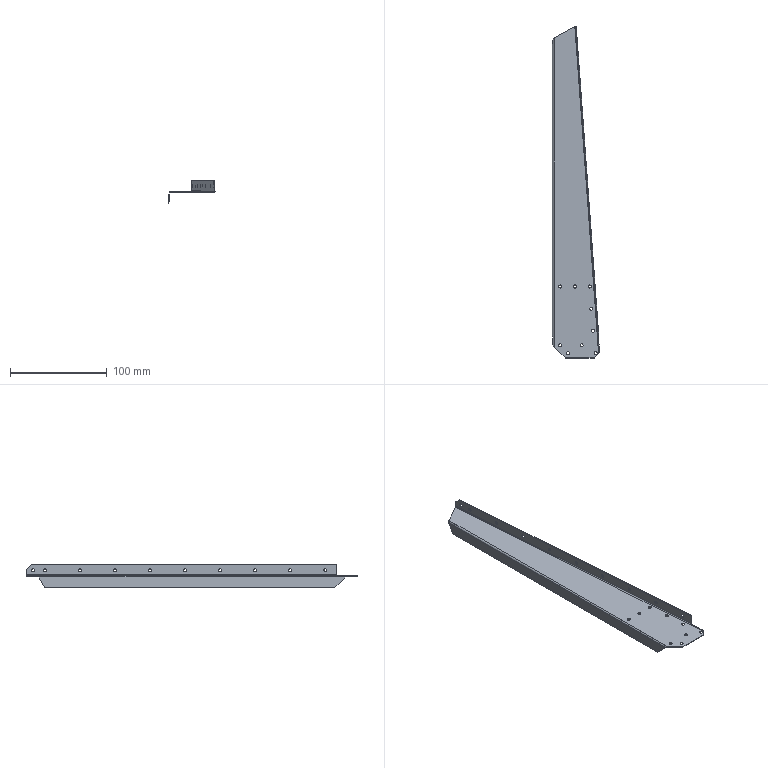Part | SolidWorks | features BaseBody 1 | 1 solid | 67 faces | box 48.846 x 343.705 x 24.041 mm | volume 9610 mm3 | cylinder 44 | plane 18 | spline 5 | commonest cylinder face diameters 3.2 x38 2 x3 3 x3